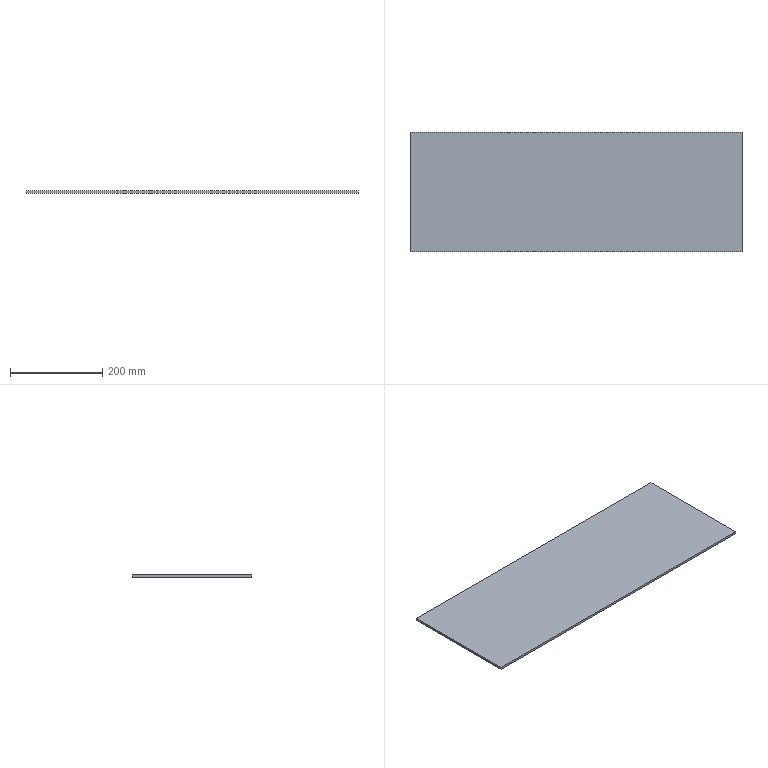Part | SolidWorks | features Extrusion 1 | 1 solid | 6 faces | box 720 x 260 x 5 mm | volume 936000 mm3 | plane 6
STEP:
#1=CARTESIAN_POINT('',(360.,-130.,0.));
#2=VERTEX_POINT('',#1);
#3=CARTESIAN_POINT('',(360.,130.,0.));
#4=VERTEX_POINT('',#3);
#5=CARTESIAN_POINT('',(360.,-130.,0.));
#6=DIRECTION('',(0.,1.,0.));
#7=VECTOR('',#6,1000.);
#8=LINE('',#5,#7);
#9=EDGE_CURVE('',#2,#4,#8,.T.);
#10=ORIENTED_EDGE('',*,*,#9,.T.);
#11=CARTESIAN_POINT('',(360.,130.,5.));
#12=VERTEX_POINT('',#11);
#13=CARTESIAN_POINT('',(360.,130.,5.));
#14=DIRECTION('',(0.,0.,-1.));
#15=VECTOR('',#14,1000.);
#16=LINE('',#13,#15);
#17=EDGE_CURVE('',#12,#4,#16,.T.);
#18=ORIENTED_EDGE('',*,*,#17,.F.);
#19=CARTESIAN_POINT('',(360.,-130.,5.));
#20=VERTEX_POINT('',#19);
#21=CARTESIAN_POINT('',(360.,-130.,5.));
#22=DIRECTION('',(0.,1.,0.));
#23=VECTOR('',#22,1000.);
#24=LINE('',#21,#23);
#25=EDGE_CURVE('',#20,#12,#24,.T.);
#26=ORIENTED_EDGE('',*,*,#25,.F.);
#27=CARTESIAN_POINT('',(360.,-130.,5.));
#28=DIRECTION('',(0.,0.,-1.));
#29=VECTOR('',#28,1000.);
#30=LINE('',#27,#29);
#31=EDGE_CURVE('',#20,#2,#30,.T.);
#32=ORIENTED_EDGE('',*,*,#31,.T.);
#33=EDGE_LOOP('',(#10,#18,#26,#32));
#34=FACE_OUTER_BOUND('',#33,.T.);
#35=CARTESIAN_POINT('',(360.,-130.,5.));
#36=DIRECTION('',(-1.,0.,0.));
#37=DIRECTION('',(0.,0.,1.));
#38=AXIS2_PLACEMENT_3D('',#35,#36,#37);
#39=PLANE('',#38);
#40=ADVANCED_FACE('',(#34),#39,.F.);
#41=CARTESIAN_POINT('',(-360.,130.,0.));
#42=VERTEX_POINT('',#41);
#43=CARTESIAN_POINT('',(-360.,130.,0.));
#44=DIRECTION('',(-1.,0.,0.));
#45=VECTOR('',#44,1000.);
#46=LINE('',#43,#45);
#47=EDGE_CURVE('',#4,#42,#46,.T.);
#48=ORIENTED_EDGE('',*,*,#47,.T.);
#49=CARTESIAN_POINT('',(-360.,130.,5.));
#50=VERTEX_POINT('',#49);
#51=CARTESIAN_POINT('',(-360.,130.,5.));
#52=DIRECTION('',(0.,0.,-1.));
#53=VECTOR('',#52,1000.);
#54=LINE('',#51,#53);
#55=EDGE_CURVE('',#50,#42,#54,.T.);
#56=ORIENTED_EDGE('',*,*,#55,.F.);
#57=CARTESIAN_POINT('',(-360.,130.,5.));
#58=DIRECTION('',(-1.,0.,0.));
#59=VECTOR('',#58,1000.);
#60=LINE('',#57,#59);
#61=EDGE_CURVE('',#12,#50,#60,.T.);
#62=ORIENTED_EDGE('',*,*,#61,.F.);
#63=ORIENTED_EDGE('',*,*,#17,.T.);
#64=EDGE_LOOP('',(#48,#56,#62,#63));
#65=FACE_OUTER_BOUND('',#64,.T.);
#66=CARTESIAN_POINT('',(-360.,130.,5.));
#67=DIRECTION('',(0.,-1.,0.));
#68=DIRECTION('',(0.,0.,-1.));
#69=AXIS2_PLACEMENT_3D('',#66,#67,#68);
#70=PLANE('',#69);
#71=ADVANCED_FACE('',(#65),#70,.F.);
#72=CARTESIAN_POINT('',(-360.,-130.,0.));
#73=VERTEX_POINT('',#72);
#74=CARTESIAN_POINT('',(-360.,-130.,0.));
#75=DIRECTION('',(0.,-1.,0.));
#76=VECTOR('',#75,1000.);
#77=LINE('',#74,#76);
#78=EDGE_CURVE('',#42,#73,#77,.T.);
#79=ORIENTED_EDGE('',*,*,#78,.T.);
#80=CARTESIAN_POINT('',(-360.,-130.,5.));
#81=VERTEX_POINT('',#80);
#82=CARTESIAN_POINT('',(-360.,-130.,5.));
#83=DIRECTION('',(0.,0.,-1.));
#84=VECTOR('',#83,1000.);
#85=LINE('',#82,#84);
#86=EDGE_CURVE('',#81,#73,#85,.T.);
#87=ORIENTED_EDGE('',*,*,#86,.F.);
#88=CARTESIAN_POINT('',(-360.,-130.,5.));
#89=DIRECTION('',(0.,-1.,0.));
#90=VECTOR('',#89,1000.);
#91=LINE('',#88,#90);
#92=EDGE_CURVE('',#50,#81,#91,.T.);
#93=ORIENTED_EDGE('',*,*,#92,.F.);
#94=ORIENTED_EDGE('',*,*,#55,.T.);
#95=EDGE_LOOP('',(#79,#87,#93,#94));
#96=FACE_OUTER_BOUND('',#95,.T.);
#97=CARTESIAN_POINT('',(-360.,-130.,5.));
#98=DIRECTION('',(1.,0.,0.));
#99=DIRECTION('',(0.,0.,-1.));
#100=AXIS2_PLACEMENT_3D('',#97,#98,#99);
#101=PLANE('',#100);
#102=ADVANCED_FACE('',(#96),#101,.F.);
#103=CARTESIAN_POINT('',(-360.,-130.,0.));
#104=DIRECTION('',(1.,0.,0.));
#105=VECTOR('',#104,1000.);
#106=LINE('',#103,#105);
#107=EDGE_CURVE('',#73,#2,#106,.T.);
#108=ORIENTED_EDGE('',*,*,#107,.T.);
#109=ORIENTED_EDGE('',*,*,#31,.F.);
#110=CARTESIAN_POINT('',(-360.,-130.,5.));
#111=DIRECTION('',(1.,0.,0.));
#112=VECTOR('',#111,1000.);
#113=LINE('',#110,#112);
#114=EDGE_CURVE('',#81,#20,#113,.T.);
#115=ORIENTED_EDGE('',*,*,#114,.F.);
#116=ORIENTED_EDGE('',*,*,#86,.T.);
#117=EDGE_LOOP('',(#108,#109,#115,#116));
#118=FACE_OUTER_BOUND('',#117,.T.);
#119=CARTESIAN_POINT('',(-360.,-130.,5.));
#120=DIRECTION('',(0.,1.,0.));
#121=DIRECTION('',(0.,0.,1.));
#122=AXIS2_PLACEMENT_3D('',#119,#120,#121);
#123=PLANE('',#122);
#124=ADVANCED_FACE('',(#118),#123,.F.);
#125=ORIENTED_EDGE('',*,*,#25,.T.);
#126=ORIENTED_EDGE('',*,*,#61,.T.);
#127=ORIENTED_EDGE('',*,*,#92,.T.);
#128=ORIENTED_EDGE('',*,*,#114,.T.);
#129=EDGE_LOOP('',(#125,#126,#127,#128));
#130=FACE_OUTER_BOUND('',#129,.T.);
#131=CARTESIAN_POINT('',(0.,0.,5.));
#132=DIRECTION('',(0.,0.,-1.));
#133=DIRECTION('',(-1.,0.,0.));
#134=AXIS2_PLACEMENT_3D('',#131,#132,#133);
#135=PLANE('',#134);
#136=ADVANCED_FACE('',(#130),#135,.F.);
#137=ORIENTED_EDGE('',*,*,#9,.F.);
#138=ORIENTED_EDGE('',*,*,#107,.F.);
#139=ORIENTED_EDGE('',*,*,#78,.F.);
#140=ORIENTED_EDGE('',*,*,#47,.F.);
#141=EDGE_LOOP('',(#137,#138,#139,#140));
#142=FACE_OUTER_BOUND('',#141,.T.);
#143=CARTESIAN_POINT('',(0.,0.,0.));
#144=DIRECTION('',(0.,0.,-1.));
#145=DIRECTION('',(-1.,0.,0.));
#146=AXIS2_PLACEMENT_3D('',#143,#144,#145);
#147=PLANE('',#146);
#148=ADVANCED_FACE('',(#142),#147,.T.);
#149=CLOSED_SHELL('',(#40,#71,#102,#124,#136,#148));
#150=MANIFOLD_SOLID_BREP('',#149);
#151=CARTESIAN_POINT('',(0.,0.,0.));
#152=DIRECTION('',(0.,0.,1.));
#153=DIRECTION('',(1.,0.,0.));
#154=AXIS2_PLACEMENT_3D('',#151,#152,#153);
#155=(LENGTH_UNIT()NAMED_UNIT(*)SI_UNIT(.MILLI.,.METRE.));
#156=UNCERTAINTY_MEASURE_WITH_UNIT(LENGTH_MEASURE(0.00001),#155,'','');
#157=(NAMED_UNIT(*)PLANE_ANGLE_UNIT()SI_UNIT($,.RADIAN.));
#158=(NAMED_UNIT(*)SI_UNIT($,.STERADIAN.)SOLID_ANGLE_UNIT());
#159=(GEOMETRIC_REPRESENTATION_CONTEXT(3)GLOBAL_UNCERTAINTY_ASSIGNED_CONTEXT((#156))GLOBAL_UNIT_ASSIGNED_CONTEXT((#155,#157,#158))REPRESENTATION_CONTEXT('',''));
#160=ADVANCED_BREP_SHAPE_REPRESENTATION('',(#150,#154),#159);